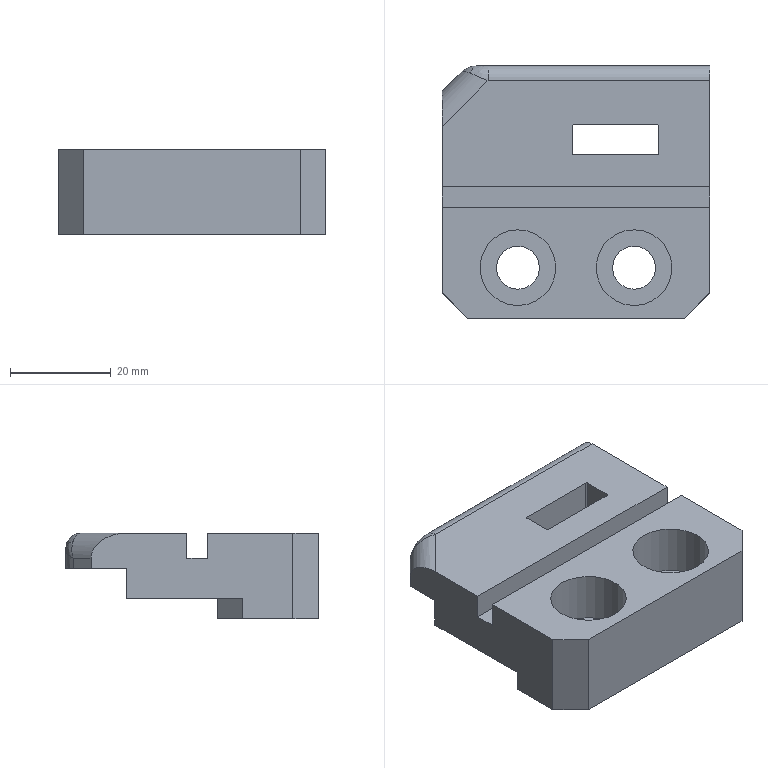Part | STEP file | gslz 2016.10.28-13_id330_x_t | 1 solid | 39 faces | box 53 x 50 x 17 mm | volume 27443 mm3 | plane 26 | cylinder 11 | spline 2 | commonest cylinder face diameters 0.6 x4 8.5 x2 10 x2 15 x2 6 x1